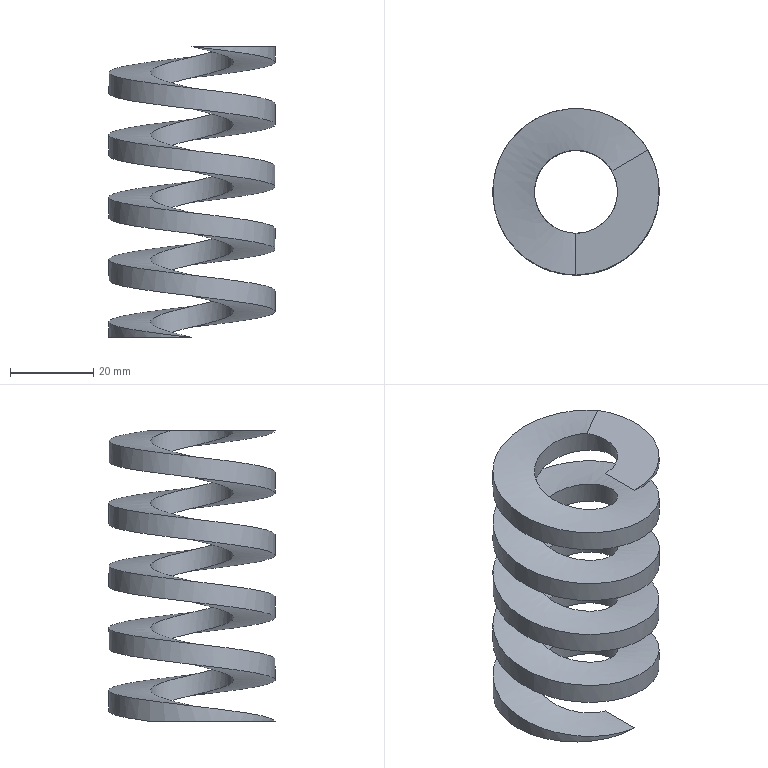Part | NX | features solid 2 | 1 solid | 6 faces | box 40 x 40.001 x 70 mm | volume 22021 mm3 | plane 2 | spline 2 | cylinder 2 | commonest cylinder face diameters 20 x1 40 x1
STEP:
#1=CARTESIAN_POINT('',(832.321,-145.002,320.));
#2=VERTEX_POINT('',#1);
#3=CARTESIAN_POINT('',(823.661,-150.001,320.));
#4=VERTEX_POINT('',#3);
#5=CARTESIAN_POINT('',(832.321,-145.002,320.));
#6=CARTESIAN_POINT('',(829.435,-146.668,320.));
#7=CARTESIAN_POINT('',(826.548,-148.334,320.));
#8=CARTESIAN_POINT('',(823.661,-150.001,320.));
#9=B_SPLINE_CURVE_WITH_KNOTS('',3,(#5,#6,#7,#8),.UNSPECIFIED.,.F.,.F.,(4,4),(0.08118,0.09118),.UNSPECIFIED.);
#10=EDGE_CURVE('',#2,#4,#9,.T.);
#11=ORIENTED_EDGE('',*,*,#10,.T.);
#12=CARTESIAN_POINT('',(815.,-165.,320.));
#13=VERTEX_POINT('',#12);
#14=CARTESIAN_POINT('',(815.,-155.,320.));
#15=DIRECTION('',(0.,0.,-1.));
#16=DIRECTION('',(0.,-1.,0.));
#17=AXIS2_PLACEMENT_3D('',#14,#15,#16);
#18=CIRCLE('',#17,10.);
#19=EDGE_CURVE('',#4,#13,#18,.T.);
#20=ORIENTED_EDGE('',*,*,#19,.T.);
#21=CARTESIAN_POINT('',(815.,-175.,320.));
#22=VERTEX_POINT('',#21);
#23=CARTESIAN_POINT('',(815.,-175.,320.));
#24=CARTESIAN_POINT('',(815.,-171.667,320.));
#25=CARTESIAN_POINT('',(815.,-168.333,320.));
#26=CARTESIAN_POINT('',(815.,-165.,320.));
#27=B_SPLINE_CURVE_WITH_KNOTS('',3,(#23,#24,#25,#26),.UNSPECIFIED.,.F.,.F.,(4,4),(0.08083,0.09083),.UNSPECIFIED.);
#28=EDGE_CURVE('',#22,#13,#27,.T.);
#29=ORIENTED_EDGE('',*,*,#28,.F.);
#30=CARTESIAN_POINT('',(815.,-155.,320.));
#31=DIRECTION('',(0.,0.,-1.));
#32=DIRECTION('',(0.,-1.,0.));
#33=AXIS2_PLACEMENT_3D('',#30,#31,#32);
#34=CIRCLE('',#33,20.);
#35=EDGE_CURVE('',#22,#2,#34,.F.);
#36=ORIENTED_EDGE('',*,*,#35,.T.);
#37=EDGE_LOOP('',(#11,#20,#29,#36));
#38=FACE_BOUND('',#37,.T.);
#39=CARTESIAN_POINT('',(815.001,-95.,320.));
#40=DIRECTION('',(0.,0.,1.));
#41=DIRECTION('',(0.,1.,0.));
#42=AXIS2_PLACEMENT_3D('',#39,#40,#41);
#43=PLANE('',#42);
#44=ADVANCED_FACE('',(#38),#43,.T.);
#45=CARTESIAN_POINT('',(797.681,-144.998,250.));
#46=VERTEX_POINT('',#45);
#47=CARTESIAN_POINT('',(806.341,-149.999,250.));
#48=VERTEX_POINT('',#47);
#49=CARTESIAN_POINT('',(797.681,-144.998,250.));
#50=DIRECTION('',(0.866,-0.5001,0.));
#51=VECTOR('',#50,1000.);
#52=LINE('',#49,#51);
#53=EDGE_CURVE('',#46,#48,#52,.T.);
#54=ORIENTED_EDGE('',*,*,#53,.T.);
#55=CARTESIAN_POINT('',(815.,-165.,250.));
#56=VERTEX_POINT('',#55);
#57=CARTESIAN_POINT('',(815.,-155.,250.));
#58=DIRECTION('',(0.,0.,1.));
#59=DIRECTION('',(0.,1.,0.));
#60=AXIS2_PLACEMENT_3D('',#57,#58,#59);
#61=CIRCLE('',#60,10.);
#62=EDGE_CURVE('',#48,#56,#61,.T.);
#63=ORIENTED_EDGE('',*,*,#62,.T.);
#64=CARTESIAN_POINT('',(815.,-175.,250.));
#65=VERTEX_POINT('',#64);
#66=CARTESIAN_POINT('',(815.,-175.,250.));
#67=DIRECTION('',(0.00004081,1.,0.));
#68=VECTOR('',#67,1000.);
#69=LINE('',#66,#68);
#70=EDGE_CURVE('',#65,#56,#69,.T.);
#71=ORIENTED_EDGE('',*,*,#70,.F.);
#72=CARTESIAN_POINT('',(815.,-155.,250.));
#73=DIRECTION('',(0.,0.,1.));
#74=DIRECTION('',(0.,1.,0.));
#75=AXIS2_PLACEMENT_3D('',#72,#73,#74);
#76=CIRCLE('',#75,20.);
#77=EDGE_CURVE('',#65,#46,#76,.F.);
#78=ORIENTED_EDGE('',*,*,#77,.T.);
#79=EDGE_LOOP('',(#54,#63,#71,#78));
#80=FACE_BOUND('',#79,.T.);
#81=CARTESIAN_POINT('',(815.001,-100.,250.));
#82=DIRECTION('',(0.,0.,-1.));
#83=DIRECTION('',(0.,-1.,0.));
#84=AXIS2_PLACEMENT_3D('',#81,#82,#83);
#85=PLANE('',#84);
#86=ADVANCED_FACE('',(#80),#85,.T.);
#87=CARTESIAN_POINT('',(797.681,-144.998,250.));
#88=CARTESIAN_POINT('',(799.223,-142.328,250.368));
#89=CARTESIAN_POINT('',(803.497,-137.785,251.094));
#90=CARTESIAN_POINT('',(812.288,-134.464,252.187));
#91=CARTESIAN_POINT('',(821.664,-135.387,253.282));
#92=CARTESIAN_POINT('',(829.649,-140.362,254.376));
#93=CARTESIAN_POINT('',(834.609,-148.33,255.467));
#94=CARTESIAN_POINT('',(835.536,-157.713,256.564));
#95=CARTESIAN_POINT('',(832.216,-166.508,257.657));
#96=CARTESIAN_POINT('',(825.369,-172.931,258.748));
#97=CARTESIAN_POINT('',(816.344,-175.67,259.845));
#98=CARTESIAN_POINT('',(807.075,-174.132,260.938));
#99=CARTESIAN_POINT('',(799.436,-168.668,262.03));
#100=CARTESIAN_POINT('',(794.989,-160.35,263.126));
#101=CARTESIAN_POINT('',(794.689,-150.964,264.218));
#102=CARTESIAN_POINT('',(798.558,-142.401,265.311));
#103=CARTESIAN_POINT('',(805.849,-136.418,266.408));
#104=CARTESIAN_POINT('',(814.992,-134.291,267.499));
#105=CARTESIAN_POINT('',(824.152,-136.417,268.592));
#106=CARTESIAN_POINT('',(831.438,-142.399,269.689));
#107=CARTESIAN_POINT('',(835.309,-150.948,270.78));
#108=CARTESIAN_POINT('',(835.011,-160.353,271.874));
#109=CARTESIAN_POINT('',(830.567,-168.661,272.97));
#110=CARTESIAN_POINT('',(822.94,-174.128,274.061));
#111=CARTESIAN_POINT('',(813.649,-175.671,275.156));
#112=CARTESIAN_POINT('',(804.642,-172.934,276.25));
#113=CARTESIAN_POINT('',(797.789,-166.522,277.342));
#114=CARTESIAN_POINT('',(794.462,-157.704,278.438));
#115=CARTESIAN_POINT('',(795.39,-148.343,279.531));
#116=CARTESIAN_POINT('',(800.34,-140.368,280.622));
#117=CARTESIAN_POINT('',(808.344,-135.384,281.719));
#118=CARTESIAN_POINT('',(817.699,-134.468,282.812));
#119=CARTESIAN_POINT('',(826.49,-137.766,283.904));
#120=CARTESIAN_POINT('',(832.941,-144.646,285.));
#121=CARTESIAN_POINT('',(835.663,-153.638,286.093));
#122=CARTESIAN_POINT('',(834.145,-162.907,287.185));
#123=CARTESIAN_POINT('',(828.654,-170.576,288.282));
#124=CARTESIAN_POINT('',(820.371,-175.,289.374));
#125=CARTESIAN_POINT('',(810.979,-175.32,290.466));
#126=CARTESIAN_POINT('',(802.388,-171.43,291.563));
#127=CARTESIAN_POINT('',(796.434,-164.174,292.654));
#128=CARTESIAN_POINT('',(794.285,-155.018,293.748));
#129=CARTESIAN_POINT('',(796.425,-145.838,294.844));
#130=CARTESIAN_POINT('',(802.377,-138.582,295.935));
#131=CARTESIAN_POINT('',(810.945,-134.686,297.029));
#132=CARTESIAN_POINT('',(820.359,-134.995,298.125));
#133=CARTESIAN_POINT('',(828.638,-139.414,299.216));
#134=CARTESIAN_POINT('',(834.134,-147.064,300.312));
#135=CARTESIAN_POINT('',(835.666,-156.35,301.406));
#136=CARTESIAN_POINT('',(832.95,-165.334,302.497));
#137=CARTESIAN_POINT('',(826.514,-172.22,303.593));
#138=CARTESIAN_POINT('',(817.711,-175.531,304.687));
#139=CARTESIAN_POINT('',(808.368,-174.622,305.778));
#140=CARTESIAN_POINT('',(800.356,-169.65,306.874));
#141=CARTESIAN_POINT('',(795.394,-161.668,307.967));
#142=CARTESIAN_POINT('',(794.46,-152.324,309.059));
#143=CARTESIAN_POINT('',(797.775,-143.494,310.156));
#144=CARTESIAN_POINT('',(804.632,-137.074,311.248));
#145=CARTESIAN_POINT('',(813.617,-134.332,312.34));
#146=CARTESIAN_POINT('',(822.924,-135.862,313.437));
#147=CARTESIAN_POINT('',(830.556,-141.331,314.529));
#148=CARTESIAN_POINT('',(835.002,-149.613,315.622));
#149=CARTESIAN_POINT('',(835.315,-159.037,316.718));
#150=CARTESIAN_POINT('',(831.446,-167.588,317.81));
#151=CARTESIAN_POINT('',(824.175,-173.566,318.904));
#152=CARTESIAN_POINT('',(818.084,-175.,319.632));
#153=CARTESIAN_POINT('',(815.,-175.,320.));
#154=B_SPLINE_CURVE_WITH_KNOTS('',3,(#87,#88,#89,#90,#91,#92,#93,#94,#95,#96,#97,#98,#99,#100,#101,#102,#103,#104,#105,#106,#107,#108,#109,#110,#111,#112,#113,#114,#115,#116,#117,#118,#119,#120,#121,#122,#123,#124,#125,#126,#127,#128,#129,#130,#131,#132,#133,#134,#135,#136,#137,#138,#139,#140,#141,#142,#143,#144,#145,#146,#147,#148,#149,#150,#151,#152,#153),.UNSPECIFIED.,.F.,.F.,(4,1,1,1,1,1,1,1,1,1,1,1,1,1,1,1,1,1,1,1,1,1,1,1,1,1,1,1,1,1,1,1,1,1,1,1,1,1,1,1,1,1,1,1,1,1,1,1,1,1,1,1,1,1,1,1,1,1,1,1,1,1,1,1,4),(0.,0.009184,0.01837,0.02755,0.03674,0.04592,0.0551,0.06429,0.07347,0.08266,0.09184,0.101,0.1102,0.1194,0.1286,0.1378,0.1469,0.1561,0.1653,0.1745,0.1837,0.1929,0.202,0.2112,0.2204,0.2296,0.2388,0.248,0.2572,0.2663,0.2755,0.2847,0.2939,0.3031,0.3123,0.3214,0.3306,0.3398,0.349,0.3582,0.3674,0.3765,0.3857,0.3949,0.4041,0.4133,0.4225,0.4316,0.4408,0.45,0.4592,0.4684,0.4776,0.4868,0.4959,0.5051,0.5143,0.5235,0.5327,0.5419,0.551,0.5602,0.5694,0.5786,0.5878),.UNSPECIFIED.);
#155=EDGE_CURVE('',#46,#22,#154,.T.);
#156=ORIENTED_EDGE('',*,*,#155,.T.);
#157=ORIENTED_EDGE('',*,*,#28,.T.);
#158=CARTESIAN_POINT('',(806.341,-149.999,250.));
#159=CARTESIAN_POINT('',(807.883,-147.329,250.736));
#160=CARTESIAN_POINT('',(812.074,-144.572,251.821));
#161=CARTESIAN_POINT('',(818.33,-145.193,253.281));
#162=CARTESIAN_POINT('',(822.327,-147.681,254.376));
#163=CARTESIAN_POINT('',(824.805,-151.669,255.468));
#164=CARTESIAN_POINT('',(825.269,-156.348,256.562));
#165=CARTESIAN_POINT('',(823.608,-160.758,257.658));
#166=CARTESIAN_POINT('',(820.18,-163.966,258.749));
#167=CARTESIAN_POINT('',(815.684,-165.334,259.842));
#168=CARTESIAN_POINT('',(811.032,-164.566,260.939));
#169=CARTESIAN_POINT('',(807.217,-161.829,262.031));
#170=CARTESIAN_POINT('',(804.998,-157.688,263.123));
#171=CARTESIAN_POINT('',(804.843,-152.975,264.22));
#172=CARTESIAN_POINT('',(806.785,-148.698,265.312));
#173=CARTESIAN_POINT('',(810.412,-145.715,266.404));
#174=CARTESIAN_POINT('',(815.003,-144.643,267.5));
#175=CARTESIAN_POINT('',(819.579,-145.713,268.593));
#176=CARTESIAN_POINT('',(823.211,-148.688,269.685));
#177=CARTESIAN_POINT('',(825.159,-152.98,270.782));
#178=CARTESIAN_POINT('',(825.002,-157.68,271.875));
#179=CARTESIAN_POINT('',(822.793,-161.818,272.967));
#180=CARTESIAN_POINT('',(817.69,-165.501,274.428));
#181=CARTESIAN_POINT('',(809.267,-164.968,276.247));
#182=CARTESIAN_POINT('',(803.596,-156.5,278.438));
#183=CARTESIAN_POINT('',(806.866,-146.875,280.623));
#184=CARTESIAN_POINT('',(816.491,-143.595,282.811));
#185=CARTESIAN_POINT('',(824.959,-149.25,285.));
#186=CARTESIAN_POINT('',(825.627,-159.388,287.185));
#187=CARTESIAN_POINT('',(817.986,-166.108,289.373));
#188=CARTESIAN_POINT('',(808.002,-164.123,291.563));
#189=CARTESIAN_POINT('',(803.502,-155.015,293.746));
#190=CARTESIAN_POINT('',(807.992,-145.879,295.936));
#191=CARTESIAN_POINT('',(817.972,-143.893,298.124));
#192=CARTESIAN_POINT('',(825.618,-150.584,300.309));
#193=CARTESIAN_POINT('',(824.964,-160.745,302.498));
#194=CARTESIAN_POINT('',(816.51,-166.398,304.686));
#195=CARTESIAN_POINT('',(806.88,-163.144,306.871));
#196=CARTESIAN_POINT('',(803.597,-153.505,309.062));
#197=CARTESIAN_POINT('',(809.239,-145.051,311.246));
#198=CARTESIAN_POINT('',(819.386,-144.367,313.434));
#199=CARTESIAN_POINT('',(826.109,-152.018,315.623));
#200=CARTESIAN_POINT('',(824.121,-161.982,317.81));
#201=CARTESIAN_POINT('',(818.084,-165.,319.264));
#202=CARTESIAN_POINT('',(815.,-165.,320.));
#203=B_SPLINE_CURVE_WITH_KNOTS('',3,(#158,#159,#160,#161,#162,#163,#164,#165,#166,#167,#168,#169,#170,#171,#172,#173,#174,#175,#176,#177,#178,#179,#180,#181,#182,#183,#184,#185,#186,#187,#188,#189,#190,#191,#192,#193,#194,#195,#196,#197,#198,#199,#200,#201,#202),.UNSPECIFIED.,.F.,.F.,(4,1,1,1,1,1,1,1,1,1,1,1,1,1,1,1,1,1,1,1,1,1,1,1,1,1,1,1,1,1,1,1,1,1,1,1,1,1,1,1,1,1,4),(0.,0.009375,0.01406,0.01875,0.02344,0.02813,0.03281,0.0375,0.04219,0.04688,0.05156,0.05625,0.06094,0.06563,0.07032,0.075,0.07969,0.08438,0.08907,0.09375,0.09844,0.1031,0.1125,0.1219,0.1313,0.1406,0.15,0.1594,0.1688,0.1781,0.1875,0.1969,0.2063,0.2156,0.225,0.2344,0.2438,0.2531,0.2625,0.2719,0.2813,0.2906,0.3),.UNSPECIFIED.);
#204=EDGE_CURVE('',#48,#13,#203,.T.);
#205=ORIENTED_EDGE('',*,*,#204,.F.);
#206=ORIENTED_EDGE('',*,*,#53,.F.);
#207=EDGE_LOOP('',(#156,#157,#205,#206));
#208=FACE_BOUND('',#207,.T.);
#209=CARTESIAN_POINT('',(806.393,-150.029,250.));
#210=CARTESIAN_POINT('',(804.241,-148.787,250.));
#211=CARTESIAN_POINT('',(802.098,-147.549,250.));
#212=CARTESIAN_POINT('',(802.011,-147.499,250.));
#213=CARTESIAN_POINT('',(797.628,-144.968,250.));
#214=CARTESIAN_POINT('',(806.966,-149.038,250.275));
#215=CARTESIAN_POINT('',(804.957,-147.548,250.275));
#216=CARTESIAN_POINT('',(802.956,-146.063,250.275));
#217=CARTESIAN_POINT('',(802.874,-146.003,250.275));
#218=CARTESIAN_POINT('',(798.783,-142.967,250.275));
#219=CARTESIAN_POINT('',(807.681,-148.129,250.55));
#220=CARTESIAN_POINT('',(805.851,-146.411,250.55));
#221=CARTESIAN_POINT('',(804.029,-144.7,250.55));
#222=CARTESIAN_POINT('',(803.954,-144.63,250.55));
#223=CARTESIAN_POINT('',(800.227,-141.132,250.55));
#224=CARTESIAN_POINT('',(808.525,-147.328,250.826));
#225=CARTESIAN_POINT('',(806.906,-145.41,250.826));
#226=CARTESIAN_POINT('',(805.293,-143.5,250.826));
#227=CARTESIAN_POINT('',(805.227,-143.422,250.826));
#228=CARTESIAN_POINT('',(801.93,-139.516,250.826));
#229=CARTESIAN_POINT('',(812.446,-144.566,251.966));
#230=CARTESIAN_POINT('',(811.807,-141.957,251.966));
#231=CARTESIAN_POINT('',(811.171,-139.359,251.966));
#232=CARTESIAN_POINT('',(811.145,-139.253,251.966));
#233=CARTESIAN_POINT('',(809.844,-133.94,251.966));
#234=CARTESIAN_POINT('',(817.652,-144.33,253.106));
#235=CARTESIAN_POINT('',(818.314,-141.663,253.106));
#236=CARTESIAN_POINT('',(818.974,-139.006,253.106));
#237=CARTESIAN_POINT('',(819.001,-138.898,253.106));
#238=CARTESIAN_POINT('',(820.351,-133.465,253.106));
#239=CARTESIAN_POINT('',(821.409,-146.066,253.961));
#240=CARTESIAN_POINT('',(823.011,-143.833,253.961));
#241=CARTESIAN_POINT('',(824.606,-141.609,253.961));
#242=CARTESIAN_POINT('',(824.671,-141.518,253.961));
#243=CARTESIAN_POINT('',(827.934,-136.969,253.961));
#244=CARTESIAN_POINT('',(826.325,-152.403,255.716));
#245=CARTESIAN_POINT('',(829.156,-151.753,255.716));
#246=CARTESIAN_POINT('',(831.975,-151.106,255.716));
#247=CARTESIAN_POINT('',(832.09,-151.08,255.716));
#248=CARTESIAN_POINT('',(837.856,-149.758,255.716));
#249=CARTESIAN_POINT('',(824.711,-160.301,257.47));
#250=CARTESIAN_POINT('',(827.139,-161.626,257.47));
#251=CARTESIAN_POINT('',(829.557,-162.946,257.47));
#252=CARTESIAN_POINT('',(829.655,-163.,257.47));
#253=CARTESIAN_POINT('',(834.6,-165.699,257.47));
#254=CARTESIAN_POINT('',(821.956,-163.603,258.349));
#255=CARTESIAN_POINT('',(823.695,-165.754,258.349));
#256=CARTESIAN_POINT('',(825.427,-167.896,258.349));
#257=CARTESIAN_POINT('',(825.498,-167.983,258.349));
#258=CARTESIAN_POINT('',(829.039,-172.364,258.349));
#259=CARTESIAN_POINT('',(814.497,-166.597,260.099));
#260=CARTESIAN_POINT('',(814.371,-169.497,260.099));
#261=CARTESIAN_POINT('',(814.245,-172.384,260.099));
#262=CARTESIAN_POINT('',(814.24,-172.502,260.099));
#263=CARTESIAN_POINT('',(813.983,-178.407,260.099));
#264=CARTESIAN_POINT('',(807.401,-162.926,261.849));
#265=CARTESIAN_POINT('',(805.501,-164.908,261.849));
#266=CARTESIAN_POINT('',(803.609,-166.882,261.849));
#267=CARTESIAN_POINT('',(803.532,-166.962,261.849));
#268=CARTESIAN_POINT('',(799.663,-170.998,261.849));
#269=CARTESIAN_POINT('',(805.02,-159.579,262.699));
#270=CARTESIAN_POINT('',(802.525,-160.724,262.699));
#271=CARTESIAN_POINT('',(800.04,-161.864,262.699));
#272=CARTESIAN_POINT('',(799.938,-161.911,262.699));
#273=CARTESIAN_POINT('',(794.857,-164.242,262.699));
#274=CARTESIAN_POINT('',(803.893,-151.766,264.428));
#275=CARTESIAN_POINT('',(801.116,-150.957,264.428));
#276=CARTESIAN_POINT('',(798.351,-150.152,264.428));
#277=CARTESIAN_POINT('',(798.238,-150.119,264.428));
#278=CARTESIAN_POINT('',(792.582,-148.473,264.428));
#279=CARTESIAN_POINT('',(809.031,-145.751,266.157));
#280=CARTESIAN_POINT('',(807.538,-143.439,266.157));
#281=CARTESIAN_POINT('',(806.052,-141.137,266.157));
#282=CARTESIAN_POINT('',(805.991,-141.043,266.157));
#283=CARTESIAN_POINT('',(802.951,-136.334,266.157));
#284=CARTESIAN_POINT('',(812.9,-144.194,267.016));
#285=CARTESIAN_POINT('',(812.375,-141.493,267.016));
#286=CARTESIAN_POINT('',(811.852,-138.802,267.016));
#287=CARTESIAN_POINT('',(811.831,-138.692,267.016));
#288=CARTESIAN_POINT('',(810.762,-133.191,267.016));
#289=CARTESIAN_POINT('',(820.705,-144.967,268.731));
#290=CARTESIAN_POINT('',(822.131,-142.458,268.731));
#291=CARTESIAN_POINT('',(823.551,-139.96,268.731));
#292=CARTESIAN_POINT('',(823.609,-139.858,268.731));
#293=CARTESIAN_POINT('',(826.513,-134.75,268.731));
#294=CARTESIAN_POINT('',(825.292,-151.28,270.445));
#295=CARTESIAN_POINT('',(827.865,-150.35,270.445));
#296=CARTESIAN_POINT('',(830.427,-149.423,270.445));
#297=CARTESIAN_POINT('',(830.532,-149.386,270.445));
#298=CARTESIAN_POINT('',(835.772,-147.491,270.445));
#299=CARTESIAN_POINT('',(825.941,-155.245,271.28));
#300=CARTESIAN_POINT('',(828.676,-155.306,271.28));
#301=CARTESIAN_POINT('',(831.4,-155.367,271.28));
#302=CARTESIAN_POINT('',(831.511,-155.37,271.28));
#303=CARTESIAN_POINT('',(837.082,-155.494,271.28));
#304=CARTESIAN_POINT('',(823.613,-162.668,272.99));
#305=CARTESIAN_POINT('',(825.766,-164.585,272.99));
#306=CARTESIAN_POINT('',(827.91,-166.495,272.99));
#307=CARTESIAN_POINT('',(827.998,-166.573,272.99));
#308=CARTESIAN_POINT('',(832.382,-170.477,272.99));
#309=CARTESIAN_POINT('',(816.499,-165.892,274.699));
#310=CARTESIAN_POINT('',(816.873,-168.615,274.699));
#311=CARTESIAN_POINT('',(817.246,-171.326,274.699));
#312=CARTESIAN_POINT('',(817.261,-171.437,274.699));
#313=CARTESIAN_POINT('',(818.024,-176.983,274.699));
#314=CARTESIAN_POINT('',(812.365,-165.674,275.553));
#315=CARTESIAN_POINT('',(811.706,-168.342,275.553));
#316=CARTESIAN_POINT('',(811.05,-171.,275.553));
#317=CARTESIAN_POINT('',(811.023,-171.108,275.553));
#318=CARTESIAN_POINT('',(809.682,-176.543,275.553));
#319=CARTESIAN_POINT('',(805.64,-161.725,277.26));
#320=CARTESIAN_POINT('',(803.299,-163.407,277.26));
#321=CARTESIAN_POINT('',(800.969,-165.081,277.26));
#322=CARTESIAN_POINT('',(800.873,-165.15,277.26));
#323=CARTESIAN_POINT('',(796.107,-168.574,277.26));
#324=CARTESIAN_POINT('',(804.1,-154.115,278.966));
#325=CARTESIAN_POINT('',(801.374,-153.894,278.966));
#326=CARTESIAN_POINT('',(798.66,-153.673,278.966));
#327=CARTESIAN_POINT('',(798.55,-153.664,278.966));
#328=CARTESIAN_POINT('',(792.999,-153.214,278.966));
#329=CARTESIAN_POINT('',(805.148,-150.252,279.799));
#330=CARTESIAN_POINT('',(802.685,-149.065,279.799));
#331=CARTESIAN_POINT('',(800.232,-147.882,279.799));
#332=CARTESIAN_POINT('',(800.132,-147.834,279.799));
#333=CARTESIAN_POINT('',(795.116,-145.417,279.799));
#334=CARTESIAN_POINT('',(810.456,-144.318,281.549));
#335=CARTESIAN_POINT('',(809.32,-141.647,281.549));
#336=CARTESIAN_POINT('',(808.188,-138.987,281.549));
#337=CARTESIAN_POINT('',(808.142,-138.879,281.549));
#338=CARTESIAN_POINT('',(805.828,-133.44,281.549));
#339=CARTESIAN_POINT('',(818.52,-144.462,283.299));
#340=CARTESIAN_POINT('',(819.4,-141.827,283.299));
#341=CARTESIAN_POINT('',(820.277,-139.204,283.299));
#342=CARTESIAN_POINT('',(820.312,-139.097,283.299));
#343=CARTESIAN_POINT('',(822.104,-133.731,283.299));
#344=CARTESIAN_POINT('',(822.342,-146.661,284.194));
#345=CARTESIAN_POINT('',(824.178,-144.576,284.194));
#346=CARTESIAN_POINT('',(826.005,-142.5,284.194));
#347=CARTESIAN_POINT('',(826.08,-142.415,284.194));
#348=CARTESIAN_POINT('',(829.818,-138.169,284.194));
#349=CARTESIAN_POINT('',(826.54,-153.593,285.952));
#350=CARTESIAN_POINT('',(829.425,-153.242,285.952));
#351=CARTESIAN_POINT('',(832.298,-152.891,285.952));
#352=CARTESIAN_POINT('',(832.415,-152.877,285.952));
#353=CARTESIAN_POINT('',(838.29,-152.161,285.952));
#354=CARTESIAN_POINT('',(824.034,-161.204,287.71));
#355=CARTESIAN_POINT('',(826.292,-162.755,287.71));
#356=CARTESIAN_POINT('',(828.541,-164.299,287.71));
#357=CARTESIAN_POINT('',(828.633,-164.362,287.71));
#358=CARTESIAN_POINT('',(833.232,-167.521,287.71));
#359=CARTESIAN_POINT('',(821.16,-164.063,288.551));
#360=CARTESIAN_POINT('',(822.7,-166.329,288.551));
#361=CARTESIAN_POINT('',(824.234,-168.585,288.551));
#362=CARTESIAN_POINT('',(824.296,-168.677,288.551));
#363=CARTESIAN_POINT('',(827.432,-173.292,288.551));
#364=CARTESIAN_POINT('',(813.668,-166.49,290.279));
#365=CARTESIAN_POINT('',(813.335,-169.362,290.279));
#366=CARTESIAN_POINT('',(813.003,-172.223,290.279));
#367=CARTESIAN_POINT('',(812.99,-172.34,290.279));
#368=CARTESIAN_POINT('',(812.311,-178.19,290.279));
#369=CARTESIAN_POINT('',(806.863,-162.443,292.007));
#370=CARTESIAN_POINT('',(804.829,-164.304,292.007));
#371=CARTESIAN_POINT('',(802.803,-166.158,292.007));
#372=CARTESIAN_POINT('',(802.72,-166.233,292.007));
#373=CARTESIAN_POINT('',(798.576,-170.023,292.007));
#374=CARTESIAN_POINT('',(804.663,-158.842,292.874));
#375=CARTESIAN_POINT('',(802.079,-159.803,292.874));
#376=CARTESIAN_POINT('',(799.505,-160.76,292.874));
#377=CARTESIAN_POINT('',(799.4,-160.799,292.874));
#378=CARTESIAN_POINT('',(794.137,-162.755,292.874));
#379=CARTESIAN_POINT('',(804.162,-150.817,294.629));
#380=CARTESIAN_POINT('',(801.452,-149.771,294.629));
#381=CARTESIAN_POINT('',(798.753,-148.729,294.629));
#382=CARTESIAN_POINT('',(798.643,-148.687,294.629));
#383=CARTESIAN_POINT('',(793.124,-146.557,294.629));
#384=CARTESIAN_POINT('',(809.925,-145.209,296.384));
#385=CARTESIAN_POINT('',(808.656,-142.761,296.384));
#386=CARTESIAN_POINT('',(807.392,-140.323,296.384));
#387=CARTESIAN_POINT('',(807.341,-140.224,296.384));
#388=CARTESIAN_POINT('',(804.756,-135.238,296.384));
#389=CARTESIAN_POINT('',(813.974,-144.019,297.251));
#390=CARTESIAN_POINT('',(813.717,-141.274,297.251));
#391=CARTESIAN_POINT('',(813.461,-138.54,297.251));
#392=CARTESIAN_POINT('',(813.451,-138.428,297.251));
#393=CARTESIAN_POINT('',(812.927,-132.838,297.251));
#394=CARTESIAN_POINT('',(821.78,-145.603,298.99));
#395=CARTESIAN_POINT('',(823.475,-143.254,298.99));
#396=CARTESIAN_POINT('',(825.163,-140.915,298.99));
#397=CARTESIAN_POINT('',(825.232,-140.819,298.99));
#398=CARTESIAN_POINT('',(828.684,-136.035,298.99));
#399=CARTESIAN_POINT('',(825.7,-152.508,300.728));
#400=CARTESIAN_POINT('',(828.375,-151.885,300.728));
#401=CARTESIAN_POINT('',(831.038,-151.265,300.728));
#402=CARTESIAN_POINT('',(831.147,-151.24,300.728));
#403=CARTESIAN_POINT('',(836.595,-149.971,300.728));
#404=CARTESIAN_POINT('',(825.865,-156.623,301.58));
#405=CARTESIAN_POINT('',(828.582,-157.029,301.58));
#406=CARTESIAN_POINT('',(831.287,-157.433,301.58));
#407=CARTESIAN_POINT('',(831.397,-157.45,301.58));
#408=CARTESIAN_POINT('',(836.929,-158.276,301.58));
#409=CARTESIAN_POINT('',(822.517,-163.814,303.317));
#410=CARTESIAN_POINT('',(824.396,-166.018,303.317));
#411=CARTESIAN_POINT('',(826.267,-168.213,303.317));
#412=CARTESIAN_POINT('',(826.343,-168.302,303.317));
#413=CARTESIAN_POINT('',(830.17,-172.79,303.317));
#414=CARTESIAN_POINT('',(814.873,-166.023,305.054));
#415=CARTESIAN_POINT('',(814.842,-168.779,305.054));
#416=CARTESIAN_POINT('',(814.81,-171.524,305.054));
#417=CARTESIAN_POINT('',(814.809,-171.636,305.054));
#418=CARTESIAN_POINT('',(814.744,-177.249,305.054));
#419=CARTESIAN_POINT('',(810.75,-165.172,305.919));
#420=CARTESIAN_POINT('',(809.688,-167.715,305.919));
#421=CARTESIAN_POINT('',(808.63,-170.248,305.919));
#422=CARTESIAN_POINT('',(808.586,-170.351,305.919));
#423=CARTESIAN_POINT('',(806.422,-175.53,305.919));
#424=CARTESIAN_POINT('',(804.581,-160.094,307.663));
#425=CARTESIAN_POINT('',(801.976,-161.367,307.663));
#426=CARTESIAN_POINT('',(799.382,-162.636,307.663));
#427=CARTESIAN_POINT('',(799.276,-162.687,307.663));
#428=CARTESIAN_POINT('',(793.971,-165.281,307.663));
#429=CARTESIAN_POINT('',(804.38,-152.118,309.408));
#430=CARTESIAN_POINT('',(801.725,-151.397,309.408));
#431=CARTESIAN_POINT('',(799.08,-150.68,309.408));
#432=CARTESIAN_POINT('',(798.973,-150.65,309.408));
#433=CARTESIAN_POINT('',(793.565,-149.183,309.408));
#434=CARTESIAN_POINT('',(806.211,-148.378,310.266));
#435=CARTESIAN_POINT('',(804.014,-146.723,310.266));
#436=CARTESIAN_POINT('',(801.825,-145.074,310.266));
#437=CARTESIAN_POINT('',(801.736,-145.007,310.266));
#438=CARTESIAN_POINT('',(797.261,-141.635,310.266));
#439=CARTESIAN_POINT('',(812.742,-143.567,312.04));
#440=CARTESIAN_POINT('',(812.177,-140.709,312.04));
#441=CARTESIAN_POINT('',(811.614,-137.862,312.04));
#442=CARTESIAN_POINT('',(811.592,-137.746,312.04));
#443=CARTESIAN_POINT('',(810.441,-131.925,312.04));
#444=CARTESIAN_POINT('',(820.689,-145.465,313.813));
#445=CARTESIAN_POINT('',(822.111,-143.081,313.813));
#446=CARTESIAN_POINT('',(823.528,-140.707,313.813));
#447=CARTESIAN_POINT('',(823.585,-140.61,313.813));
#448=CARTESIAN_POINT('',(826.482,-135.755,313.813));
#449=CARTESIAN_POINT('',(823.942,-148.417,314.706));
#450=CARTESIAN_POINT('',(826.177,-146.771,314.706));
#451=CARTESIAN_POINT('',(828.403,-145.132,314.706));
#452=CARTESIAN_POINT('',(828.494,-145.065,314.706));
#453=CARTESIAN_POINT('',(833.046,-141.714,314.706));
#454=CARTESIAN_POINT('',(826.344,-155.403,316.309));
#455=CARTESIAN_POINT('',(829.179,-155.504,316.309));
#456=CARTESIAN_POINT('',(832.004,-155.604,316.309));
#457=CARTESIAN_POINT('',(832.119,-155.608,316.309));
#458=CARTESIAN_POINT('',(837.894,-155.814,316.309));
#459=CARTESIAN_POINT('',(823.175,-161.766,317.913));
#460=CARTESIAN_POINT('',(825.219,-163.458,317.913));
#461=CARTESIAN_POINT('',(827.254,-165.142,317.913));
#462=CARTESIAN_POINT('',(827.337,-165.211,317.913));
#463=CARTESIAN_POINT('',(831.499,-168.656,317.913));
#464=CARTESIAN_POINT('',(820.802,-163.879,318.606));
#465=CARTESIAN_POINT('',(822.253,-166.099,318.606));
#466=CARTESIAN_POINT('',(823.697,-168.309,318.606));
#467=CARTESIAN_POINT('',(823.756,-168.399,318.606));
#468=CARTESIAN_POINT('',(826.71,-172.92,318.606));
#469=CARTESIAN_POINT('',(817.905,-164.939,319.302));
#470=CARTESIAN_POINT('',(818.631,-167.424,319.302));
#471=CARTESIAN_POINT('',(819.354,-169.899,319.302));
#472=CARTESIAN_POINT('',(819.383,-170.,319.302));
#473=CARTESIAN_POINT('',(820.862,-175.061,319.302));
#474=CARTESIAN_POINT('',(815.,-164.939,320.));
#475=CARTESIAN_POINT('',(815.,-167.424,320.));
#476=CARTESIAN_POINT('',(815.,-169.899,320.));
#477=CARTESIAN_POINT('',(815.,-170.,320.));
#478=CARTESIAN_POINT('',(815.,-175.061,320.));
#479=B_SPLINE_SURFACE_WITH_KNOTS('',5,1,((#209,#210,#211,#212,#213),(#214,#215,#216,#217,#218),(#219,#220,#221,#222,#223),(#224,#225,#226,#227,#228),(#229,#230,#231,#232,#233),(#234,#235,#236,#237,#238),(#239,#240,#241,#242,#243),(#244,#245,#246,#247,#248),(#249,#250,#251,#252,#253),(#254,#255,#256,#257,#258),(#259,#260,#261,#262,#263),(#264,#265,#266,#267,#268),(#269,#270,#271,#272,#273),(#274,#275,#276,#277,#278),(#279,#280,#281,#282,#283),(#284,#285,#286,#287,#288),(#289,#290,#291,#292,#293),(#294,#295,#296,#297,#298),(#299,#300,#301,#302,#303),(#304,#305,#306,#307,#308),(#309,#310,#311,#312,#313),(#314,#315,#316,#317,#318),(#319,#320,#321,#322,#323),(#324,#325,#326,#327,#328),(#329,#330,#331,#332,#333),(#334,#335,#336,#337,#338),(#339,#340,#341,#342,#343),(#344,#345,#346,#347,#348),(#349,#350,#351,#352,#353),(#354,#355,#356,#357,#358),(#359,#360,#361,#362,#363),(#364,#365,#366,#367,#368),(#369,#370,#371,#372,#373),(#374,#375,#376,#377,#378),(#379,#380,#381,#382,#383),(#384,#385,#386,#387,#388),(#389,#390,#391,#392,#393),(#394,#395,#396,#397,#398),(#399,#400,#401,#402,#403),(#404,#405,#406,#407,#408),(#409,#410,#411,#412,#413),(#414,#415,#416,#417,#418),(#419,#420,#421,#422,#423),(#424,#425,#426,#427,#428),(#429,#430,#431,#432,#433),(#434,#435,#436,#437,#438),(#439,#440,#441,#442,#443),(#444,#445,#446,#447,#448),(#449,#450,#451,#452,#453),(#454,#455,#456,#457,#458),(#459,#460,#461,#462,#463),(#464,#465,#466,#467,#468),(#469,#470,#471,#472,#473),(#474,#475,#476,#477,#478)),.RULED_SURF.,.F.,.F.,.F.,(6,3,3,3,3,3,3,3,3,3,3,3,3,3,3,3,3,6),(2,1,1,1,2),(0.3125,0.316,0.3267,0.3378,0.3485,0.3594,0.3699,0.3807,0.3912,0.4025,0.4131,0.4241,0.435,0.4458,0.4567,0.4675,0.4788,0.4875),(-0.5061,-0.2576,-0.0101,0.,0.5061),.UNSPECIFIED.);
#480=ADVANCED_FACE('',(#208),#479,.F.);
#481=ORIENTED_EDGE('',*,*,#35,.F.);
#482=ORIENTED_EDGE('',*,*,#155,.F.);
#483=ORIENTED_EDGE('',*,*,#77,.F.);
#484=CARTESIAN_POINT('',(815.,-175.,250.));
#485=CARTESIAN_POINT('',(811.916,-175.,250.368));
#486=CARTESIAN_POINT('',(805.844,-173.57,251.093));
#487=CARTESIAN_POINT('',(798.573,-167.618,252.186));
#488=CARTESIAN_POINT('',(794.683,-159.037,253.282));
#489=CARTESIAN_POINT('',(794.998,-149.634,254.376));
#490=CARTESIAN_POINT('',(799.418,-141.354,255.467));
#491=CARTESIAN_POINT('',(807.08,-135.859,256.563));
#492=CARTESIAN_POINT('',(816.357,-134.336,257.657));
#493=CARTESIAN_POINT('',(825.343,-137.054,258.748));
#494=CARTESIAN_POINT('',(832.228,-143.5,259.845));
#495=CARTESIAN_POINT('',(835.531,-152.296,260.937));
#496=CARTESIAN_POINT('',(834.619,-161.644,262.03));
#497=CARTESIAN_POINT('',(829.64,-169.654,263.126));
#498=CARTESIAN_POINT('',(821.661,-174.608,264.218));
#499=CARTESIAN_POINT('',(812.311,-175.539,265.311));
#500=CARTESIAN_POINT('',(803.485,-172.217,266.408));
#501=CARTESIAN_POINT('',(797.07,-165.362,267.499));
#502=CARTESIAN_POINT('',(794.331,-156.367,268.592));
#503=CARTESIAN_POINT('',(795.868,-147.066,269.688));
#504=CARTESIAN_POINT('',(801.336,-139.438,270.78));
#505=CARTESIAN_POINT('',(809.63,-134.993,271.874));
#506=CARTESIAN_POINT('',(819.047,-134.688,272.969));
#507=CARTESIAN_POINT('',(827.595,-138.56,274.061));
#508=CARTESIAN_POINT('',(833.577,-145.834,275.156));
#509=CARTESIAN_POINT('',(835.71,-155.003,276.25));
#510=CARTESIAN_POINT('',(833.584,-164.144,277.342));
#511=CARTESIAN_POINT('',(827.611,-171.434,278.438));
#512=CARTESIAN_POINT('',(819.041,-175.311,279.532));
#513=CARTESIAN_POINT('',(809.659,-175.012,280.622));
#514=CARTESIAN_POINT('',(801.34,-170.572,281.719));
#515=CARTESIAN_POINT('',(795.869,-162.929,282.812));
#516=CARTESIAN_POINT('',(794.33,-153.666,283.904));
#517=CARTESIAN_POINT('',(797.063,-144.64,285.));
#518=CARTESIAN_POINT('',(803.488,-137.786,286.093));
#519=CARTESIAN_POINT('',(812.275,-134.466,287.185));
#520=CARTESIAN_POINT('',(821.662,-135.387,288.282));
#521=CARTESIAN_POINT('',(829.635,-140.349,289.373));
#522=CARTESIAN_POINT('',(834.609,-148.323,290.466));
#523=CARTESIAN_POINT('',(835.535,-157.707,291.563));
#524=CARTESIAN_POINT('',(832.227,-166.492,292.655));
#525=CARTESIAN_POINT('',(825.372,-172.931,293.748));
#526=CARTESIAN_POINT('',(816.352,-175.668,294.844));
#527=CARTESIAN_POINT('',(807.092,-174.141,295.935));
#528=CARTESIAN_POINT('',(799.435,-168.668,297.03));
#529=CARTESIAN_POINT('',(794.995,-160.361,298.125));
#530=CARTESIAN_POINT('',(794.683,-150.981,299.216));
#531=CARTESIAN_POINT('',(798.56,-142.397,300.311));
#532=CARTESIAN_POINT('',(805.837,-136.428,301.406));
#533=CARTESIAN_POINT('',(814.975,-134.288,302.497));
#534=CARTESIAN_POINT('',(824.157,-136.419,303.593));
#535=CARTESIAN_POINT('',(831.425,-142.388,304.687));
#536=CARTESIAN_POINT('',(835.31,-150.933,305.778));
#537=CARTESIAN_POINT('',(835.009,-160.359,306.874));
#538=CARTESIAN_POINT('',(830.577,-168.646,307.968));
#539=CARTESIAN_POINT('',(822.952,-174.126,309.06));
#540=CARTESIAN_POINT('',(813.647,-175.67,310.156));
#541=CARTESIAN_POINT('',(804.658,-172.941,311.248));
#542=CARTESIAN_POINT('',(797.792,-166.53,312.341));
#543=CARTESIAN_POINT('',(794.464,-157.705,313.437));
#544=CARTESIAN_POINT('',(795.385,-148.361,314.529));
#545=CARTESIAN_POINT('',(800.335,-140.37,315.622));
#546=CARTESIAN_POINT('',(808.34,-135.388,316.719));
#547=CARTESIAN_POINT('',(817.68,-134.463,317.81));
#548=CARTESIAN_POINT('',(826.493,-137.772,318.905));
#549=CARTESIAN_POINT('',(830.78,-142.331,319.632));
#550=CARTESIAN_POINT('',(832.321,-145.002,320.));
#551=B_SPLINE_CURVE_WITH_KNOTS('',3,(#484,#485,#486,#487,#488,#489,#490,#491,#492,#493,#494,#495,#496,#497,#498,#499,#500,#501,#502,#503,#504,#505,#506,#507,#508,#509,#510,#511,#512,#513,#514,#515,#516,#517,#518,#519,#520,#521,#522,#523,#524,#525,#526,#527,#528,#529,#530,#531,#532,#533,#534,#535,#536,#537,#538,#539,#540,#541,#542,#543,#544,#545,#546,#547,#548,#549,#550),.UNSPECIFIED.,.F.,.F.,(4,1,1,1,1,1,1,1,1,1,1,1,1,1,1,1,1,1,1,1,1,1,1,1,1,1,1,1,1,1,1,1,1,1,1,1,1,1,1,1,1,1,1,1,1,1,1,1,1,1,1,1,1,1,1,1,1,1,1,1,1,1,1,1,4),(0.,0.009184,0.01837,0.02755,0.03674,0.04592,0.0551,0.06429,0.07347,0.08266,0.09184,0.101,0.1102,0.1194,0.1286,0.1378,0.1469,0.1561,0.1653,0.1745,0.1837,0.1929,0.202,0.2112,0.2204,0.2296,0.2388,0.248,0.2572,0.2663,0.2755,0.2847,0.2939,0.3031,0.3123,0.3214,0.3306,0.3398,0.349,0.3582,0.3674,0.3765,0.3857,0.3949,0.4041,0.4133,0.4225,0.4317,0.4408,0.45,0.4592,0.4684,0.4776,0.4868,0.4959,0.5051,0.5143,0.5235,0.5327,0.5419,0.551,0.5602,0.5694,0.5786,0.5878),.UNSPECIFIED.);
#552=EDGE_CURVE('',#65,#2,#551,.T.);
#553=ORIENTED_EDGE('',*,*,#552,.T.);
#554=EDGE_LOOP('',(#481,#482,#483,#553));
#555=FACE_BOUND('',#554,.T.);
#556=CARTESIAN_POINT('',(815.,-155.,208.997));
#557=DIRECTION('',(0.,0.,1.));
#558=DIRECTION('',(0.,1.,0.));
#559=AXIS2_PLACEMENT_3D('',#556,#557,#558);
#560=CYLINDRICAL_SURFACE('',#559,20.);
#561=ADVANCED_FACE('',(#555),#560,.T.);
#562=CARTESIAN_POINT('',(815.,-165.,250.));
#563=CARTESIAN_POINT('',(811.917,-165.,250.736));
#564=CARTESIAN_POINT('',(807.434,-162.749,251.821));
#565=CARTESIAN_POINT('',(804.843,-157.021,253.281));
#566=CARTESIAN_POINT('',(804.998,-152.315,254.376));
#567=CARTESIAN_POINT('',(807.213,-148.175,255.468));
#568=CARTESIAN_POINT('',(811.032,-145.433,256.561));
#569=CARTESIAN_POINT('',(815.682,-144.666,257.658));
#570=CARTESIAN_POINT('',(820.175,-146.031,258.749));
#571=CARTESIAN_POINT('',(823.608,-149.24,259.842));
#572=CARTESIAN_POINT('',(825.269,-153.653,260.939));
#573=CARTESIAN_POINT('',(824.806,-158.325,262.031));
#574=CARTESIAN_POINT('',(822.33,-162.318,263.123));
#575=CARTESIAN_POINT('',(818.326,-164.808,264.22));
#576=CARTESIAN_POINT('',(813.651,-165.266,265.312));
#577=CARTESIAN_POINT('',(809.254,-163.616,266.404));
#578=CARTESIAN_POINT('',(806.03,-160.176,267.5));
#579=CARTESIAN_POINT('',(804.668,-155.679,268.593));
#580=CARTESIAN_POINT('',(805.429,-151.046,269.685));
#581=CARTESIAN_POINT('',(808.172,-147.213,270.782));
#582=CARTESIAN_POINT('',(812.32,-144.998,271.874));
#583=CARTESIAN_POINT('',(817.008,-144.843,272.966));
#584=CARTESIAN_POINT('',(822.75,-147.42,274.428));
#585=CARTESIAN_POINT('',(826.5,-154.981,276.247));
#586=CARTESIAN_POINT('',(822.002,-164.126,278.438));
#587=CARTESIAN_POINT('',(812.032,-166.107,280.623));
#588=CARTESIAN_POINT('',(804.378,-159.411,282.81));
#589=CARTESIAN_POINT('',(805.042,-149.25,285.));
#590=CARTESIAN_POINT('',(813.487,-143.602,287.185));
#591=CARTESIAN_POINT('',(823.127,-146.86,289.373));
#592=CARTESIAN_POINT('',(826.4,-156.499,291.563));
#593=CARTESIAN_POINT('',(820.762,-164.95,293.746));
#594=CARTESIAN_POINT('',(810.606,-165.63,295.936));
#595=CARTESIAN_POINT('',(803.895,-157.98,298.124));
#596=CARTESIAN_POINT('',(805.867,-148.013,300.309));
#597=CARTESIAN_POINT('',(814.994,-143.498,302.498));
#598=CARTESIAN_POINT('',(824.116,-147.994,304.686));
#599=CARTESIAN_POINT('',(826.113,-157.961,306.871));
#600=CARTESIAN_POINT('',(819.406,-165.623,309.062));
#601=CARTESIAN_POINT('',(809.264,-164.964,311.247));
#602=CARTESIAN_POINT('',(803.599,-156.517,313.435));
#603=CARTESIAN_POINT('',(806.864,-146.87,315.623));
#604=CARTESIAN_POINT('',(816.488,-143.611,317.81));
#605=CARTESIAN_POINT('',(822.119,-147.33,319.264));
#606=CARTESIAN_POINT('',(823.661,-150.001,320.));
#607=B_SPLINE_CURVE_WITH_KNOTS('',3,(#562,#563,#564,#565,#566,#567,#568,#569,#570,#571,#572,#573,#574,#575,#576,#577,#578,#579,#580,#581,#582,#583,#584,#585,#586,#587,#588,#589,#590,#591,#592,#593,#594,#595,#596,#597,#598,#599,#600,#601,#602,#603,#604,#605,#606),.UNSPECIFIED.,.F.,.F.,(4,1,1,1,1,1,1,1,1,1,1,1,1,1,1,1,1,1,1,1,1,1,1,1,1,1,1,1,1,1,1,1,1,1,1,1,1,1,1,1,1,1,4),(0.,0.009375,0.01406,0.01875,0.02344,0.02813,0.03281,0.0375,0.04219,0.04688,0.05156,0.05625,0.06094,0.06563,0.07032,0.075,0.07969,0.08438,0.08907,0.09375,0.09844,0.1031,0.1125,0.1219,0.1313,0.1406,0.15,0.1594,0.1688,0.1781,0.1875,0.1969,0.2063,0.2156,0.225,0.2344,0.2438,0.2531,0.2625,0.2719,0.2813,0.2906,0.3),.UNSPECIFIED.);
#608=EDGE_CURVE('',#56,#4,#607,.T.);
#609=ORIENTED_EDGE('',*,*,#608,.T.);
#610=ORIENTED_EDGE('',*,*,#10,.F.);
#611=ORIENTED_EDGE('',*,*,#552,.F.);
#612=ORIENTED_EDGE('',*,*,#70,.T.);
#613=EDGE_LOOP('',(#609,#610,#611,#612));
#614=FACE_BOUND('',#613,.T.);
#615=CARTESIAN_POINT('',(815.,-175.061,250.));
#616=CARTESIAN_POINT('',(815.,-170.,250.));
#617=CARTESIAN_POINT('',(815.,-169.899,250.));
#618=CARTESIAN_POINT('',(815.,-167.424,250.));
#619=CARTESIAN_POINT('',(815.,-164.939,250.));
#620=CARTESIAN_POINT('',(811.764,-175.061,250.385));
#621=CARTESIAN_POINT('',(812.581,-170.,250.385));
#622=CARTESIAN_POINT('',(812.597,-169.899,250.385));
#623=CARTESIAN_POINT('',(812.996,-167.424,250.385));
#624=CARTESIAN_POINT('',(813.397,-164.939,250.385));
#625=CARTESIAN_POINT('',(808.527,-174.408,250.77));
#626=CARTESIAN_POINT('',(810.16,-169.512,250.77));
#627=CARTESIAN_POINT('',(810.193,-169.414,250.77));
#628=CARTESIAN_POINT('',(810.991,-167.02,250.77));
#629=CARTESIAN_POINT('',(811.793,-164.616,250.77));
#630=CARTESIAN_POINT('',(805.461,-173.102,251.156));
#631=CARTESIAN_POINT('',(807.867,-168.536,251.156));
#632=CARTESIAN_POINT('',(807.915,-168.444,251.156));
#633=CARTESIAN_POINT('',(809.092,-166.211,251.156));
#634=CARTESIAN_POINT('',(810.274,-163.969,251.156));
#635=CARTESIAN_POINT('',(796.466,-166.836,252.435));
#636=CARTESIAN_POINT('',(801.141,-163.85,252.435));
#637=CARTESIAN_POINT('',(801.235,-163.79,252.435));
#638=CARTESIAN_POINT('',(803.521,-162.33,252.435));
#639=CARTESIAN_POINT('',(805.817,-160.864,252.435));
#640=CARTESIAN_POINT('',(792.672,-155.601,253.713));
#641=CARTESIAN_POINT('',(798.305,-155.449,253.713));
#642=CARTESIAN_POINT('',(798.418,-155.446,253.713));
#643=CARTESIAN_POINT('',(801.172,-155.372,253.713));
#644=CARTESIAN_POINT('',(803.938,-155.297,253.713));
#645=CARTESIAN_POINT('',(794.136,-147.027,254.594));
#646=CARTESIAN_POINT('',(799.399,-149.039,254.594));
#647=CARTESIAN_POINT('',(799.504,-149.079,254.594));
#648=CARTESIAN_POINT('',(802.078,-150.062,254.594));
#649=CARTESIAN_POINT('',(804.663,-151.05,254.594));
#650=CARTESIAN_POINT('',(804.169,-134.197,256.35));
#651=CARTESIAN_POINT('',(806.901,-139.445,256.35));
#652=CARTESIAN_POINT('',(806.956,-139.55,256.35));
#653=CARTESIAN_POINT('',(808.292,-142.116,256.35));
#654=CARTESIAN_POINT('',(809.634,-144.693,256.35));
#655=CARTESIAN_POINT('',(820.351,-133.465,258.106));
#656=CARTESIAN_POINT('',(819.001,-138.898,258.106));
#657=CARTESIAN_POINT('',(818.974,-139.006,258.106));
#658=CARTESIAN_POINT('',(818.314,-141.663,258.106));
#659=CARTESIAN_POINT('',(817.652,-144.33,258.106));
#660=CARTESIAN_POINT('',(827.934,-136.969,258.961));
#661=CARTESIAN_POINT('',(824.671,-141.518,258.961));
#662=CARTESIAN_POINT('',(824.606,-141.609,258.961));
#663=CARTESIAN_POINT('',(823.011,-143.833,258.961));
#664=CARTESIAN_POINT('',(821.409,-146.066,258.961));
#665=CARTESIAN_POINT('',(837.856,-149.758,260.716));
#666=CARTESIAN_POINT('',(832.09,-151.08,260.716));
#667=CARTESIAN_POINT('',(831.975,-151.106,260.716));
#668=CARTESIAN_POINT('',(829.156,-151.753,260.716));
#669=CARTESIAN_POINT('',(826.325,-152.403,260.716));
#670=CARTESIAN_POINT('',(834.6,-165.699,262.47));
#671=CARTESIAN_POINT('',(829.655,-163.,262.47));
#672=CARTESIAN_POINT('',(829.557,-162.946,262.47));
#673=CARTESIAN_POINT('',(827.139,-161.626,262.47));
#674=CARTESIAN_POINT('',(824.711,-160.301,262.47));
#675=CARTESIAN_POINT('',(829.039,-172.364,263.349));
#676=CARTESIAN_POINT('',(825.498,-167.983,263.349));
#677=CARTESIAN_POINT('',(825.427,-167.896,263.349));
#678=CARTESIAN_POINT('',(823.695,-165.754,263.349));
#679=CARTESIAN_POINT('',(821.956,-163.603,263.349));
#680=CARTESIAN_POINT('',(813.983,-178.407,265.099));
#681=CARTESIAN_POINT('',(814.24,-172.502,265.099));
#682=CARTESIAN_POINT('',(814.245,-172.384,265.099));
#683=CARTESIAN_POINT('',(814.371,-169.497,265.099));
#684=CARTESIAN_POINT('',(814.497,-166.597,265.099));
#685=CARTESIAN_POINT('',(799.663,-170.998,266.849));
#686=CARTESIAN_POINT('',(803.532,-166.962,266.849));
#687=CARTESIAN_POINT('',(803.609,-166.882,266.849));
#688=CARTESIAN_POINT('',(805.501,-164.908,266.849));
#689=CARTESIAN_POINT('',(807.401,-162.926,266.849));
#690=CARTESIAN_POINT('',(794.857,-164.242,267.699));
#691=CARTESIAN_POINT('',(799.938,-161.911,267.699));
#692=CARTESIAN_POINT('',(800.04,-161.864,267.699));
#693=CARTESIAN_POINT('',(802.525,-160.724,267.699));
#694=CARTESIAN_POINT('',(805.02,-159.579,267.699));
#695=CARTESIAN_POINT('',(792.582,-148.473,269.428));
#696=CARTESIAN_POINT('',(798.238,-150.119,269.428));
#697=CARTESIAN_POINT('',(798.351,-150.152,269.428));
#698=CARTESIAN_POINT('',(801.116,-150.957,269.428));
#699=CARTESIAN_POINT('',(803.893,-151.766,269.428));
#700=CARTESIAN_POINT('',(802.951,-136.334,271.157));
#701=CARTESIAN_POINT('',(805.991,-141.043,271.157));
#702=CARTESIAN_POINT('',(806.052,-141.137,271.157));
#703=CARTESIAN_POINT('',(807.538,-143.439,271.157));
#704=CARTESIAN_POINT('',(809.031,-145.751,271.157));
#705=CARTESIAN_POINT('',(810.762,-133.191,272.016));
#706=CARTESIAN_POINT('',(811.831,-138.692,272.016));
#707=CARTESIAN_POINT('',(811.852,-138.802,272.016));
#708=CARTESIAN_POINT('',(812.375,-141.493,272.016));
#709=CARTESIAN_POINT('',(812.9,-144.194,272.016));
#710=CARTESIAN_POINT('',(826.513,-134.75,273.731));
#711=CARTESIAN_POINT('',(823.609,-139.858,273.731));
#712=CARTESIAN_POINT('',(823.551,-139.96,273.731));
#713=CARTESIAN_POINT('',(822.131,-142.458,273.731));
#714=CARTESIAN_POINT('',(820.705,-144.967,273.731));
#715=CARTESIAN_POINT('',(835.772,-147.491,275.445));
#716=CARTESIAN_POINT('',(830.532,-149.386,275.445));
#717=CARTESIAN_POINT('',(830.427,-149.423,275.445));
#718=CARTESIAN_POINT('',(827.865,-150.35,275.445));
#719=CARTESIAN_POINT('',(825.292,-151.28,275.445));
#720=CARTESIAN_POINT('',(837.082,-155.494,276.28));
#721=CARTESIAN_POINT('',(831.511,-155.37,276.28));
#722=CARTESIAN_POINT('',(831.4,-155.367,276.28));
#723=CARTESIAN_POINT('',(828.676,-155.306,276.28));
#724=CARTESIAN_POINT('',(825.941,-155.245,276.28));
#725=CARTESIAN_POINT('',(832.382,-170.477,277.99));
#726=CARTESIAN_POINT('',(827.998,-166.573,277.99));
#727=CARTESIAN_POINT('',(827.91,-166.495,277.99));
#728=CARTESIAN_POINT('',(825.766,-164.585,277.99));
#729=CARTESIAN_POINT('',(823.613,-162.668,277.99));
#730=CARTESIAN_POINT('',(818.024,-176.983,279.699));
#731=CARTESIAN_POINT('',(817.261,-171.437,279.699));
#732=CARTESIAN_POINT('',(817.246,-171.326,279.699));
#733=CARTESIAN_POINT('',(816.873,-168.615,279.699));
#734=CARTESIAN_POINT('',(816.499,-165.892,279.699));
#735=CARTESIAN_POINT('',(809.682,-176.543,280.553));
#736=CARTESIAN_POINT('',(811.023,-171.108,280.553));
#737=CARTESIAN_POINT('',(811.05,-171.,280.553));
#738=CARTESIAN_POINT('',(811.706,-168.342,280.553));
#739=CARTESIAN_POINT('',(812.365,-165.674,280.553));
#740=CARTESIAN_POINT('',(796.107,-168.574,282.26));
#741=CARTESIAN_POINT('',(800.873,-165.15,282.26));
#742=CARTESIAN_POINT('',(800.969,-165.081,282.26));
#743=CARTESIAN_POINT('',(803.299,-163.407,282.26));
#744=CARTESIAN_POINT('',(805.64,-161.725,282.26));
#745=CARTESIAN_POINT('',(792.999,-153.214,283.966));
#746=CARTESIAN_POINT('',(798.55,-153.664,283.966));
#747=CARTESIAN_POINT('',(798.66,-153.673,283.966));
#748=CARTESIAN_POINT('',(801.374,-153.894,283.966));
#749=CARTESIAN_POINT('',(804.1,-154.115,283.966));
#750=CARTESIAN_POINT('',(795.116,-145.417,284.799));
#751=CARTESIAN_POINT('',(800.132,-147.834,284.799));
#752=CARTESIAN_POINT('',(800.232,-147.882,284.799));
#753=CARTESIAN_POINT('',(802.685,-149.065,284.799));
#754=CARTESIAN_POINT('',(805.148,-150.252,284.799));
#755=CARTESIAN_POINT('',(805.828,-133.44,286.549));
#756=CARTESIAN_POINT('',(808.142,-138.879,286.549));
#757=CARTESIAN_POINT('',(808.188,-138.987,286.549));
#758=CARTESIAN_POINT('',(809.32,-141.647,286.549));
#759=CARTESIAN_POINT('',(810.456,-144.318,286.549));
#760=CARTESIAN_POINT('',(822.104,-133.731,288.299));
#761=CARTESIAN_POINT('',(820.312,-139.097,288.299));
#762=CARTESIAN_POINT('',(820.277,-139.204,288.299));
#763=CARTESIAN_POINT('',(819.4,-141.827,288.299));
#764=CARTESIAN_POINT('',(818.52,-144.462,288.299));
#765=CARTESIAN_POINT('',(829.818,-138.169,289.194));
#766=CARTESIAN_POINT('',(826.08,-142.415,289.194));
#767=CARTESIAN_POINT('',(826.005,-142.5,289.194));
#768=CARTESIAN_POINT('',(824.178,-144.576,289.194));
#769=CARTESIAN_POINT('',(822.342,-146.661,289.194));
#770=CARTESIAN_POINT('',(838.29,-152.161,290.952));
#771=CARTESIAN_POINT('',(832.415,-152.877,290.952));
#772=CARTESIAN_POINT('',(832.298,-152.891,290.952));
#773=CARTESIAN_POINT('',(829.425,-153.242,290.952));
#774=CARTESIAN_POINT('',(826.54,-153.593,290.952));
#775=CARTESIAN_POINT('',(833.232,-167.521,292.71));
#776=CARTESIAN_POINT('',(828.633,-164.362,292.71));
#777=CARTESIAN_POINT('',(828.541,-164.299,292.71));
#778=CARTESIAN_POINT('',(826.292,-162.755,292.71));
#779=CARTESIAN_POINT('',(824.034,-161.204,292.71));
#780=CARTESIAN_POINT('',(827.432,-173.292,293.551));
#781=CARTESIAN_POINT('',(824.296,-168.677,293.551));
#782=CARTESIAN_POINT('',(824.234,-168.585,293.551));
#783=CARTESIAN_POINT('',(822.7,-166.329,293.551));
#784=CARTESIAN_POINT('',(821.16,-164.063,293.551));
#785=CARTESIAN_POINT('',(812.311,-178.19,295.279));
#786=CARTESIAN_POINT('',(812.99,-172.34,295.279));
#787=CARTESIAN_POINT('',(813.003,-172.223,295.279));
#788=CARTESIAN_POINT('',(813.335,-169.362,295.279));
#789=CARTESIAN_POINT('',(813.668,-166.49,295.279));
#790=CARTESIAN_POINT('',(798.576,-170.023,297.007));
#791=CARTESIAN_POINT('',(802.72,-166.233,297.007));
#792=CARTESIAN_POINT('',(802.803,-166.158,297.007));
#793=CARTESIAN_POINT('',(804.829,-164.304,297.007));
#794=CARTESIAN_POINT('',(806.863,-162.443,297.007));
#795=CARTESIAN_POINT('',(794.137,-162.755,297.874));
#796=CARTESIAN_POINT('',(799.4,-160.799,297.874));
#797=CARTESIAN_POINT('',(799.505,-160.76,297.874));
#798=CARTESIAN_POINT('',(802.079,-159.803,297.874));
#799=CARTESIAN_POINT('',(804.663,-158.842,297.874));
#800=CARTESIAN_POINT('',(793.124,-146.557,299.629));
#801=CARTESIAN_POINT('',(798.643,-148.687,299.629));
#802=CARTESIAN_POINT('',(798.753,-148.729,299.629));
#803=CARTESIAN_POINT('',(801.452,-149.771,299.629));
#804=CARTESIAN_POINT('',(804.162,-150.817,299.629));
#805=CARTESIAN_POINT('',(804.756,-135.238,301.384));
#806=CARTESIAN_POINT('',(807.341,-140.224,301.384));
#807=CARTESIAN_POINT('',(807.392,-140.323,301.384));
#808=CARTESIAN_POINT('',(808.656,-142.761,301.384));
#809=CARTESIAN_POINT('',(809.925,-145.209,301.384));
#810=CARTESIAN_POINT('',(812.927,-132.838,302.251));
#811=CARTESIAN_POINT('',(813.451,-138.428,302.251));
#812=CARTESIAN_POINT('',(813.461,-138.54,302.251));
#813=CARTESIAN_POINT('',(813.717,-141.274,302.251));
#814=CARTESIAN_POINT('',(813.974,-144.019,302.251));
#815=CARTESIAN_POINT('',(828.684,-136.035,303.99));
#816=CARTESIAN_POINT('',(825.232,-140.819,303.99));
#817=CARTESIAN_POINT('',(825.163,-140.915,303.99));
#818=CARTESIAN_POINT('',(823.475,-143.254,303.99));
#819=CARTESIAN_POINT('',(821.78,-145.603,303.99));
#820=CARTESIAN_POINT('',(836.595,-149.971,305.728));
#821=CARTESIAN_POINT('',(831.147,-151.24,305.728));
#822=CARTESIAN_POINT('',(831.038,-151.265,305.728));
#823=CARTESIAN_POINT('',(828.375,-151.885,305.728));
#824=CARTESIAN_POINT('',(825.7,-152.508,305.728));
#825=CARTESIAN_POINT('',(836.929,-158.276,306.58));
#826=CARTESIAN_POINT('',(831.397,-157.45,306.58));
#827=CARTESIAN_POINT('',(831.287,-157.433,306.58));
#828=CARTESIAN_POINT('',(828.582,-157.029,306.58));
#829=CARTESIAN_POINT('',(825.865,-156.623,306.58));
#830=CARTESIAN_POINT('',(830.17,-172.79,308.317));
#831=CARTESIAN_POINT('',(826.343,-168.302,308.317));
#832=CARTESIAN_POINT('',(826.267,-168.213,308.317));
#833=CARTESIAN_POINT('',(824.396,-166.018,308.317));
#834=CARTESIAN_POINT('',(822.517,-163.814,308.317));
#835=CARTESIAN_POINT('',(814.744,-177.249,310.054));
#836=CARTESIAN_POINT('',(814.809,-171.636,310.054));
#837=CARTESIAN_POINT('',(814.81,-171.524,310.054));
#838=CARTESIAN_POINT('',(814.842,-168.779,310.054));
#839=CARTESIAN_POINT('',(814.873,-166.023,310.054));
#840=CARTESIAN_POINT('',(806.422,-175.53,310.919));
#841=CARTESIAN_POINT('',(808.586,-170.351,310.919));
#842=CARTESIAN_POINT('',(808.63,-170.248,310.919));
#843=CARTESIAN_POINT('',(809.688,-167.715,310.919));
#844=CARTESIAN_POINT('',(810.75,-165.172,310.919));
#845=CARTESIAN_POINT('',(793.971,-165.281,312.663));
#846=CARTESIAN_POINT('',(799.276,-162.687,312.663));
#847=CARTESIAN_POINT('',(799.382,-162.636,312.663));
#848=CARTESIAN_POINT('',(801.976,-161.367,312.663));
#849=CARTESIAN_POINT('',(804.581,-160.094,312.663));
#850=CARTESIAN_POINT('',(793.565,-149.183,314.408));
#851=CARTESIAN_POINT('',(798.973,-150.65,314.408));
#852=CARTESIAN_POINT('',(799.08,-150.68,314.408));
#853=CARTESIAN_POINT('',(801.725,-151.397,314.408));
#854=CARTESIAN_POINT('',(804.38,-152.118,314.408));
#855=CARTESIAN_POINT('',(797.261,-141.635,315.266));
#856=CARTESIAN_POINT('',(801.736,-145.007,315.266));
#857=CARTESIAN_POINT('',(801.825,-145.074,315.266));
#858=CARTESIAN_POINT('',(804.014,-146.723,315.266));
#859=CARTESIAN_POINT('',(806.211,-148.378,315.266));
#860=CARTESIAN_POINT('',(808.184,-133.588,316.736));
#861=CARTESIAN_POINT('',(809.904,-138.989,316.736));
#862=CARTESIAN_POINT('',(809.938,-139.097,316.736));
#863=CARTESIAN_POINT('',(810.779,-141.738,316.736));
#864=CARTESIAN_POINT('',(811.623,-144.391,316.736));
#865=CARTESIAN_POINT('',(821.072,-134.841,318.206));
#866=CARTESIAN_POINT('',(819.54,-139.926,318.206));
#867=CARTESIAN_POINT('',(819.51,-140.028,318.206));
#868=CARTESIAN_POINT('',(818.761,-142.514,318.206));
#869=CARTESIAN_POINT('',(818.009,-145.012,318.206));
#870=CARTESIAN_POINT('',(825.979,-137.05,318.803));
#871=CARTESIAN_POINT('',(823.21,-141.578,318.803));
#872=CARTESIAN_POINT('',(823.154,-141.668,318.803));
#873=CARTESIAN_POINT('',(821.8,-143.883,318.803));
#874=CARTESIAN_POINT('',(820.44,-146.106,318.803));
#875=CARTESIAN_POINT('',(829.859,-140.612,319.401));
#876=CARTESIAN_POINT('',(826.11,-144.242,319.401));
#877=CARTESIAN_POINT('',(826.036,-144.314,319.401));
#878=CARTESIAN_POINT('',(824.203,-146.089,319.401));
#879=CARTESIAN_POINT('',(822.362,-147.871,319.401));
#880=CARTESIAN_POINT('',(832.375,-144.971,320.));
#881=CARTESIAN_POINT('',(827.992,-147.501,320.));
#882=CARTESIAN_POINT('',(827.904,-147.551,320.));
#883=CARTESIAN_POINT('',(825.761,-148.788,320.));
#884=CARTESIAN_POINT('',(823.609,-150.031,320.));
#885=B_SPLINE_SURFACE_WITH_KNOTS('',5,1,((#615,#616,#617,#618,#619),(#620,#621,#622,#623,#624),(#625,#626,#627,#628,#629),(#630,#631,#632,#633,#634),(#635,#636,#637,#638,#639),(#640,#641,#642,#643,#644),(#645,#646,#647,#648,#649),(#650,#651,#652,#653,#654),(#655,#656,#657,#658,#659),(#660,#661,#662,#663,#664),(#665,#666,#667,#668,#669),(#670,#671,#672,#673,#674),(#675,#676,#677,#678,#679),(#680,#681,#682,#683,#684),(#685,#686,#687,#688,#689),(#690,#691,#692,#693,#694),(#695,#696,#697,#698,#699),(#700,#701,#702,#703,#704),(#705,#706,#707,#708,#709),(#710,#711,#712,#713,#714),(#715,#716,#717,#718,#719),(#720,#721,#722,#723,#724),(#725,#726,#727,#728,#729),(#730,#731,#732,#733,#734),(#735,#736,#737,#738,#739),(#740,#741,#742,#743,#744),(#745,#746,#747,#748,#749),(#750,#751,#752,#753,#754),(#755,#756,#757,#758,#759),(#760,#761,#762,#763,#764),(#765,#766,#767,#768,#769),(#770,#771,#772,#773,#774),(#775,#776,#777,#778,#779),(#780,#781,#782,#783,#784),(#785,#786,#787,#788,#789),(#790,#791,#792,#793,#794),(#795,#796,#797,#798,#799),(#800,#801,#802,#803,#804),(#805,#806,#807,#808,#809),(#810,#811,#812,#813,#814),(#815,#816,#817,#818,#819),(#820,#821,#822,#823,#824),(#825,#826,#827,#828,#829),(#830,#831,#832,#833,#834),(#835,#836,#837,#838,#839),(#840,#841,#842,#843,#844),(#845,#846,#847,#848,#849),(#850,#851,#852,#853,#854),(#855,#856,#857,#858,#859),(#860,#861,#862,#863,#864),(#865,#866,#867,#868,#869),(#870,#871,#872,#873,#874),(#875,#876,#877,#878,#879),(#880,#881,#882,#883,#884)),.RULED_SURF.,.F.,.F.,.F.,(6,3,3,3,3,3,3,3,3,3,3,3,3,3,3,3,3,6),(2,1,1,1,2),(0.3,0.3048,0.316,0.3267,0.3378,0.3485,0.3594,0.3699,0.3807,0.3912,0.4025,0.4131,0.4241,0.435,0.4458,0.4567,0.4675,0.475),(0.4939,1.,1.01,1.258,1.506),.UNSPECIFIED.);
#886=ADVANCED_FACE('',(#614),#885,.F.);
#887=ORIENTED_EDGE('',*,*,#19,.F.);
#888=ORIENTED_EDGE('',*,*,#608,.F.);
#889=ORIENTED_EDGE('',*,*,#62,.F.);
#890=ORIENTED_EDGE('',*,*,#204,.T.);
#891=EDGE_LOOP('',(#887,#888,#889,#890));
#892=FACE_BOUND('',#891,.T.);
#893=CARTESIAN_POINT('',(815.,-155.,205.997));
#894=DIRECTION('',(0.,0.,1.));
#895=DIRECTION('',(0.,1.,0.));
#896=AXIS2_PLACEMENT_3D('',#893,#894,#895);
#897=CYLINDRICAL_SURFACE('',#896,10.);
#898=ADVANCED_FACE('',(#892),#897,.F.);
#899=CLOSED_SHELL('',(#44,#86,#480,#561,#886,#898));
#900=MANIFOLD_SOLID_BREP('',#899);
#901=(LENGTH_UNIT()NAMED_UNIT(*)SI_UNIT(.MILLI.,.METRE.));
#902=UNCERTAINTY_MEASURE_WITH_UNIT(LENGTH_MEASURE(0.0508),#901,'','');
#903=(NAMED_UNIT(*)PLANE_ANGLE_UNIT()SI_UNIT($,.RADIAN.));
#904=(NAMED_UNIT(*)SI_UNIT($,.STERADIAN.)SOLID_ANGLE_UNIT());
#905=(GEOMETRIC_REPRESENTATION_CONTEXT(3)GLOBAL_UNCERTAINTY_ASSIGNED_CONTEXT((#902))GLOBAL_UNIT_ASSIGNED_CONTEXT((#901,#903,#904))REPRESENTATION_CONTEXT('',''));
#906=ADVANCED_BREP_SHAPE_REPRESENTATION('',(#900),#905);